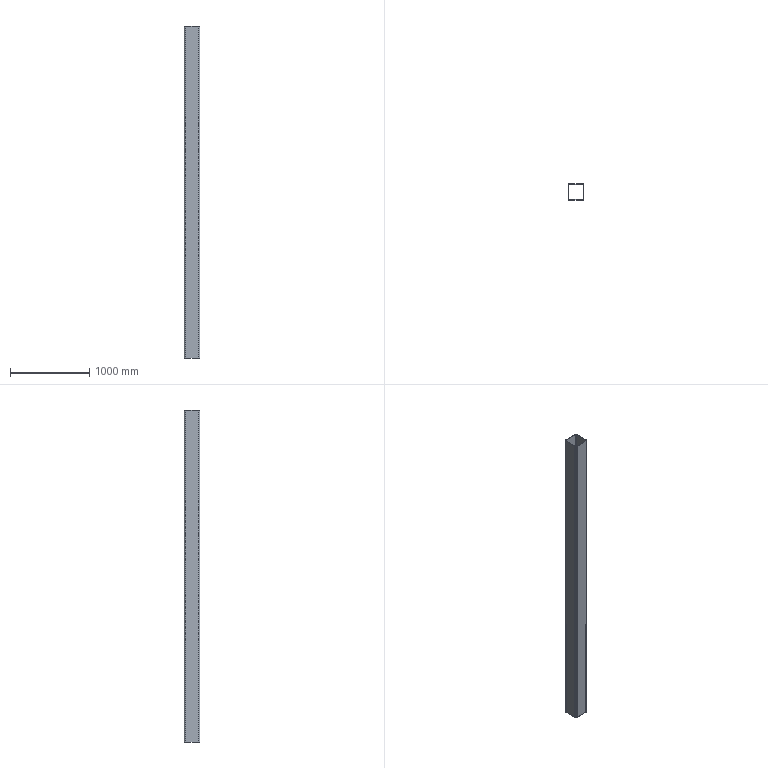Part | SolidWorks | features Extrusion 1 | 1 solid | 18 faces | box 200 x 200 x 4180 mm | volume 15674075 mm3 | plane 10 | cylinder 8 | commonest cylinder face diameters 30 x4 40 x4
STEP:
#1=CARTESIAN_POINT('',(-100.,-80.,4180.));
#2=VERTEX_POINT('',#1);
#3=CARTESIAN_POINT('',(-80.,-100.,4180.));
#4=VERTEX_POINT('',#3);
#5=CARTESIAN_POINT('',(-80.,-80.,4180.));
#6=DIRECTION('',(0.,0.,1.));
#7=DIRECTION('',(1.,0.,0.));
#8=AXIS2_PLACEMENT_3D('',#5,#6,#7);
#9=CIRCLE('',#8,20.);
#10=EDGE_CURVE('',#2,#4,#9,.T.);
#11=ORIENTED_EDGE('',*,*,#10,.T.);
#12=CARTESIAN_POINT('',(80.,-100.,4180.));
#13=VERTEX_POINT('',#12);
#14=CARTESIAN_POINT('',(-80.,-100.,4180.));
#15=DIRECTION('',(1.,0.,0.));
#16=VECTOR('',#15,1000.);
#17=LINE('',#14,#16);
#18=EDGE_CURVE('',#4,#13,#17,.T.);
#19=ORIENTED_EDGE('',*,*,#18,.T.);
#20=CARTESIAN_POINT('',(100.,-80.,4180.));
#21=VERTEX_POINT('',#20);
#22=CARTESIAN_POINT('',(80.,-80.,4180.));
#23=DIRECTION('',(0.,0.,1.));
#24=DIRECTION('',(1.,0.,0.));
#25=AXIS2_PLACEMENT_3D('',#22,#23,#24);
#26=CIRCLE('',#25,20.);
#27=EDGE_CURVE('',#13,#21,#26,.T.);
#28=ORIENTED_EDGE('',*,*,#27,.T.);
#29=CARTESIAN_POINT('',(100.,80.,4180.));
#30=VERTEX_POINT('',#29);
#31=CARTESIAN_POINT('',(100.,80.,4180.));
#32=DIRECTION('',(0.,1.,0.));
#33=VECTOR('',#32,1000.);
#34=LINE('',#31,#33);
#35=EDGE_CURVE('',#21,#30,#34,.T.);
#36=ORIENTED_EDGE('',*,*,#35,.T.);
#37=CARTESIAN_POINT('',(80.,100.,4180.));
#38=VERTEX_POINT('',#37);
#39=CARTESIAN_POINT('',(80.,80.,4180.));
#40=DIRECTION('',(0.,0.,1.));
#41=DIRECTION('',(-1.,0.,0.));
#42=AXIS2_PLACEMENT_3D('',#39,#40,#41);
#43=CIRCLE('',#42,20.);
#44=EDGE_CURVE('',#30,#38,#43,.T.);
#45=ORIENTED_EDGE('',*,*,#44,.T.);
#46=CARTESIAN_POINT('',(-80.,100.,4180.));
#47=VERTEX_POINT('',#46);
#48=CARTESIAN_POINT('',(-80.,100.,4180.));
#49=DIRECTION('',(-1.,0.,0.));
#50=VECTOR('',#49,1000.);
#51=LINE('',#48,#50);
#52=EDGE_CURVE('',#38,#47,#51,.T.);
#53=ORIENTED_EDGE('',*,*,#52,.T.);
#54=CARTESIAN_POINT('',(-100.,80.,4180.));
#55=VERTEX_POINT('',#54);
#56=CARTESIAN_POINT('',(-80.,80.,4180.));
#57=DIRECTION('',(0.,0.,1.));
#58=DIRECTION('',(1.,0.,0.));
#59=AXIS2_PLACEMENT_3D('',#56,#57,#58);
#60=CIRCLE('',#59,20.);
#61=EDGE_CURVE('',#47,#55,#60,.T.);
#62=ORIENTED_EDGE('',*,*,#61,.T.);
#63=CARTESIAN_POINT('',(-100.,80.,4180.));
#64=DIRECTION('',(0.,-1.,0.));
#65=VECTOR('',#64,1000.);
#66=LINE('',#63,#65);
#67=EDGE_CURVE('',#55,#2,#66,.T.);
#68=ORIENTED_EDGE('',*,*,#67,.T.);
#69=EDGE_LOOP('',(#11,#19,#28,#36,#45,#53,#62,#68));
#70=FACE_OUTER_BOUND('',#69,.T.);
#71=CARTESIAN_POINT('',(-95.,80.,4180.));
#72=VERTEX_POINT('',#71);
#73=CARTESIAN_POINT('',(-95.,-80.,4180.));
#74=VERTEX_POINT('',#73);
#75=CARTESIAN_POINT('',(-95.,80.,4180.));
#76=DIRECTION('',(0.,-1.,0.));
#77=VECTOR('',#76,1000.);
#78=LINE('',#75,#77);
#79=EDGE_CURVE('',#72,#74,#78,.T.);
#80=ORIENTED_EDGE('',*,*,#79,.F.);
#81=CARTESIAN_POINT('',(-80.,95.,4180.));
#82=VERTEX_POINT('',#81);
#83=CARTESIAN_POINT('',(-80.,80.,4180.));
#84=DIRECTION('',(0.,0.,1.));
#85=DIRECTION('',(1.,0.,0.));
#86=AXIS2_PLACEMENT_3D('',#83,#84,#85);
#87=CIRCLE('',#86,15.);
#88=EDGE_CURVE('',#82,#72,#87,.T.);
#89=ORIENTED_EDGE('',*,*,#88,.F.);
#90=CARTESIAN_POINT('',(80.,95.,4180.));
#91=VERTEX_POINT('',#90);
#92=CARTESIAN_POINT('',(-80.,95.,4180.));
#93=DIRECTION('',(-1.,0.,0.));
#94=VECTOR('',#93,1000.);
#95=LINE('',#92,#94);
#96=EDGE_CURVE('',#91,#82,#95,.T.);
#97=ORIENTED_EDGE('',*,*,#96,.F.);
#98=CARTESIAN_POINT('',(95.,80.,4180.));
#99=VERTEX_POINT('',#98);
#100=CARTESIAN_POINT('',(80.,80.,4180.));
#101=DIRECTION('',(0.,0.,1.));
#102=DIRECTION('',(-1.,0.,0.));
#103=AXIS2_PLACEMENT_3D('',#100,#101,#102);
#104=CIRCLE('',#103,15.);
#105=EDGE_CURVE('',#99,#91,#104,.T.);
#106=ORIENTED_EDGE('',*,*,#105,.F.);
#107=CARTESIAN_POINT('',(95.,-80.,4180.));
#108=VERTEX_POINT('',#107);
#109=CARTESIAN_POINT('',(95.,80.,4180.));
#110=DIRECTION('',(0.,1.,0.));
#111=VECTOR('',#110,1000.);
#112=LINE('',#109,#111);
#113=EDGE_CURVE('',#108,#99,#112,.T.);
#114=ORIENTED_EDGE('',*,*,#113,.F.);
#115=CARTESIAN_POINT('',(80.,-95.,4180.));
#116=VERTEX_POINT('',#115);
#117=CARTESIAN_POINT('',(80.,-80.,4180.));
#118=DIRECTION('',(0.,0.,1.));
#119=DIRECTION('',(1.,0.,0.));
#120=AXIS2_PLACEMENT_3D('',#117,#118,#119);
#121=CIRCLE('',#120,15.);
#122=EDGE_CURVE('',#116,#108,#121,.T.);
#123=ORIENTED_EDGE('',*,*,#122,.F.);
#124=CARTESIAN_POINT('',(-80.,-95.,4180.));
#125=VERTEX_POINT('',#124);
#126=CARTESIAN_POINT('',(-80.,-95.,4180.));
#127=DIRECTION('',(1.,0.,0.));
#128=VECTOR('',#127,1000.);
#129=LINE('',#126,#128);
#130=EDGE_CURVE('',#125,#116,#129,.T.);
#131=ORIENTED_EDGE('',*,*,#130,.F.);
#132=CARTESIAN_POINT('',(-80.,-80.,4180.));
#133=DIRECTION('',(0.,0.,1.));
#134=DIRECTION('',(1.,0.,0.));
#135=AXIS2_PLACEMENT_3D('',#132,#133,#134);
#136=CIRCLE('',#135,15.);
#137=EDGE_CURVE('',#74,#125,#136,.T.);
#138=ORIENTED_EDGE('',*,*,#137,.F.);
#139=EDGE_LOOP('',(#80,#89,#97,#106,#114,#123,#131,#138));
#140=FACE_BOUND('',#139,.T.);
#141=CARTESIAN_POINT('',(-80.,-80.,4180.));
#142=DIRECTION('',(0.,0.,1.));
#143=DIRECTION('',(1.,0.,0.));
#144=AXIS2_PLACEMENT_3D('',#141,#142,#143);
#145=PLANE('',#144);
#146=ADVANCED_FACE('',(#70,#140),#145,.T.);
#147=CARTESIAN_POINT('',(-100.,-80.,0.));
#148=VERTEX_POINT('',#147);
#149=CARTESIAN_POINT('',(-80.,-100.,0.));
#150=VERTEX_POINT('',#149);
#151=CARTESIAN_POINT('',(-80.,-80.,0.));
#152=DIRECTION('',(0.,0.,1.));
#153=DIRECTION('',(1.,0.,0.));
#154=AXIS2_PLACEMENT_3D('',#151,#152,#153);
#155=CIRCLE('',#154,20.);
#156=EDGE_CURVE('',#148,#150,#155,.T.);
#157=ORIENTED_EDGE('',*,*,#156,.F.);
#158=CARTESIAN_POINT('',(-100.,80.,0.));
#159=VERTEX_POINT('',#158);
#160=CARTESIAN_POINT('',(-100.,80.,0.));
#161=DIRECTION('',(0.,-1.,0.));
#162=VECTOR('',#161,1000.);
#163=LINE('',#160,#162);
#164=EDGE_CURVE('',#159,#148,#163,.T.);
#165=ORIENTED_EDGE('',*,*,#164,.F.);
#166=CARTESIAN_POINT('',(-80.,100.,0.));
#167=VERTEX_POINT('',#166);
#168=CARTESIAN_POINT('',(-80.,80.,0.));
#169=DIRECTION('',(0.,0.,1.));
#170=DIRECTION('',(1.,0.,0.));
#171=AXIS2_PLACEMENT_3D('',#168,#169,#170);
#172=CIRCLE('',#171,20.);
#173=EDGE_CURVE('',#167,#159,#172,.T.);
#174=ORIENTED_EDGE('',*,*,#173,.F.);
#175=CARTESIAN_POINT('',(80.,100.,0.));
#176=VERTEX_POINT('',#175);
#177=CARTESIAN_POINT('',(-80.,100.,0.));
#178=DIRECTION('',(-1.,0.,0.));
#179=VECTOR('',#178,1000.);
#180=LINE('',#177,#179);
#181=EDGE_CURVE('',#176,#167,#180,.T.);
#182=ORIENTED_EDGE('',*,*,#181,.F.);
#183=CARTESIAN_POINT('',(100.,80.,0.));
#184=VERTEX_POINT('',#183);
#185=CARTESIAN_POINT('',(80.,80.,0.));
#186=DIRECTION('',(0.,0.,1.));
#187=DIRECTION('',(-1.,0.,0.));
#188=AXIS2_PLACEMENT_3D('',#185,#186,#187);
#189=CIRCLE('',#188,20.);
#190=EDGE_CURVE('',#184,#176,#189,.T.);
#191=ORIENTED_EDGE('',*,*,#190,.F.);
#192=CARTESIAN_POINT('',(100.,-80.,0.));
#193=VERTEX_POINT('',#192);
#194=CARTESIAN_POINT('',(100.,80.,0.));
#195=DIRECTION('',(0.,1.,0.));
#196=VECTOR('',#195,1000.);
#197=LINE('',#194,#196);
#198=EDGE_CURVE('',#193,#184,#197,.T.);
#199=ORIENTED_EDGE('',*,*,#198,.F.);
#200=CARTESIAN_POINT('',(80.,-100.,0.));
#201=VERTEX_POINT('',#200);
#202=CARTESIAN_POINT('',(80.,-80.,0.));
#203=DIRECTION('',(0.,0.,1.));
#204=DIRECTION('',(1.,0.,0.));
#205=AXIS2_PLACEMENT_3D('',#202,#203,#204);
#206=CIRCLE('',#205,20.);
#207=EDGE_CURVE('',#201,#193,#206,.T.);
#208=ORIENTED_EDGE('',*,*,#207,.F.);
#209=CARTESIAN_POINT('',(-80.,-100.,0.));
#210=DIRECTION('',(1.,0.,0.));
#211=VECTOR('',#210,1000.);
#212=LINE('',#209,#211);
#213=EDGE_CURVE('',#150,#201,#212,.T.);
#214=ORIENTED_EDGE('',*,*,#213,.F.);
#215=EDGE_LOOP('',(#157,#165,#174,#182,#191,#199,#208,#214));
#216=FACE_OUTER_BOUND('',#215,.T.);
#217=CARTESIAN_POINT('',(-80.,95.,0.));
#218=VERTEX_POINT('',#217);
#219=CARTESIAN_POINT('',(-95.,80.,0.));
#220=VERTEX_POINT('',#219);
#221=CARTESIAN_POINT('',(-80.,80.,0.));
#222=DIRECTION('',(0.,0.,1.));
#223=DIRECTION('',(1.,0.,0.));
#224=AXIS2_PLACEMENT_3D('',#221,#222,#223);
#225=CIRCLE('',#224,15.);
#226=EDGE_CURVE('',#218,#220,#225,.T.);
#227=ORIENTED_EDGE('',*,*,#226,.T.);
#228=CARTESIAN_POINT('',(-95.,-80.,0.));
#229=VERTEX_POINT('',#228);
#230=CARTESIAN_POINT('',(-95.,80.,0.));
#231=DIRECTION('',(0.,-1.,0.));
#232=VECTOR('',#231,1000.);
#233=LINE('',#230,#232);
#234=EDGE_CURVE('',#220,#229,#233,.T.);
#235=ORIENTED_EDGE('',*,*,#234,.T.);
#236=CARTESIAN_POINT('',(-80.,-95.,0.));
#237=VERTEX_POINT('',#236);
#238=CARTESIAN_POINT('',(-80.,-80.,0.));
#239=DIRECTION('',(0.,0.,1.));
#240=DIRECTION('',(1.,0.,0.));
#241=AXIS2_PLACEMENT_3D('',#238,#239,#240);
#242=CIRCLE('',#241,15.);
#243=EDGE_CURVE('',#229,#237,#242,.T.);
#244=ORIENTED_EDGE('',*,*,#243,.T.);
#245=CARTESIAN_POINT('',(80.,-95.,0.));
#246=VERTEX_POINT('',#245);
#247=CARTESIAN_POINT('',(-80.,-95.,0.));
#248=DIRECTION('',(1.,0.,0.));
#249=VECTOR('',#248,1000.);
#250=LINE('',#247,#249);
#251=EDGE_CURVE('',#237,#246,#250,.T.);
#252=ORIENTED_EDGE('',*,*,#251,.T.);
#253=CARTESIAN_POINT('',(95.,-80.,0.));
#254=VERTEX_POINT('',#253);
#255=CARTESIAN_POINT('',(80.,-80.,0.));
#256=DIRECTION('',(0.,0.,1.));
#257=DIRECTION('',(1.,0.,0.));
#258=AXIS2_PLACEMENT_3D('',#255,#256,#257);
#259=CIRCLE('',#258,15.);
#260=EDGE_CURVE('',#246,#254,#259,.T.);
#261=ORIENTED_EDGE('',*,*,#260,.T.);
#262=CARTESIAN_POINT('',(95.,80.,0.));
#263=VERTEX_POINT('',#262);
#264=CARTESIAN_POINT('',(95.,80.,0.));
#265=DIRECTION('',(0.,1.,0.));
#266=VECTOR('',#265,1000.);
#267=LINE('',#264,#266);
#268=EDGE_CURVE('',#254,#263,#267,.T.);
#269=ORIENTED_EDGE('',*,*,#268,.T.);
#270=CARTESIAN_POINT('',(80.,95.,0.));
#271=VERTEX_POINT('',#270);
#272=CARTESIAN_POINT('',(80.,80.,0.));
#273=DIRECTION('',(0.,0.,1.));
#274=DIRECTION('',(-1.,0.,0.));
#275=AXIS2_PLACEMENT_3D('',#272,#273,#274);
#276=CIRCLE('',#275,15.);
#277=EDGE_CURVE('',#263,#271,#276,.T.);
#278=ORIENTED_EDGE('',*,*,#277,.T.);
#279=CARTESIAN_POINT('',(-80.,95.,0.));
#280=DIRECTION('',(-1.,0.,0.));
#281=VECTOR('',#280,1000.);
#282=LINE('',#279,#281);
#283=EDGE_CURVE('',#271,#218,#282,.T.);
#284=ORIENTED_EDGE('',*,*,#283,.T.);
#285=EDGE_LOOP('',(#227,#235,#244,#252,#261,#269,#278,#284));
#286=FACE_BOUND('',#285,.T.);
#287=CARTESIAN_POINT('',(-80.,-80.,0.));
#288=DIRECTION('',(0.,0.,1.));
#289=DIRECTION('',(1.,0.,0.));
#290=AXIS2_PLACEMENT_3D('',#287,#288,#289);
#291=PLANE('',#290);
#292=ADVANCED_FACE('',(#216,#286),#291,.F.);
#293=ORIENTED_EDGE('',*,*,#156,.T.);
#294=CARTESIAN_POINT('',(-80.,-100.,4180.));
#295=DIRECTION('',(0.,0.,-1.));
#296=VECTOR('',#295,1000.);
#297=LINE('',#294,#296);
#298=EDGE_CURVE('',#4,#150,#297,.T.);
#299=ORIENTED_EDGE('',*,*,#298,.F.);
#300=ORIENTED_EDGE('',*,*,#10,.F.);
#301=CARTESIAN_POINT('',(-100.,-80.,4180.));
#302=DIRECTION('',(0.,0.,-1.));
#303=VECTOR('',#302,1000.);
#304=LINE('',#301,#303);
#305=EDGE_CURVE('',#2,#148,#304,.T.);
#306=ORIENTED_EDGE('',*,*,#305,.T.);
#307=EDGE_LOOP('',(#293,#299,#300,#306));
#308=FACE_OUTER_BOUND('',#307,.T.);
#309=CARTESIAN_POINT('',(-80.,-80.,4180.));
#310=DIRECTION('',(0.,0.,-1.));
#311=DIRECTION('',(-1.,0.,0.));
#312=AXIS2_PLACEMENT_3D('',#309,#310,#311);
#313=CYLINDRICAL_SURFACE('',#312,20.);
#314=ADVANCED_FACE('',(#308),#313,.T.);
#315=ORIENTED_EDGE('',*,*,#213,.T.);
#316=CARTESIAN_POINT('',(80.,-100.,4180.));
#317=DIRECTION('',(0.,0.,-1.));
#318=VECTOR('',#317,1000.);
#319=LINE('',#316,#318);
#320=EDGE_CURVE('',#13,#201,#319,.T.);
#321=ORIENTED_EDGE('',*,*,#320,.F.);
#322=ORIENTED_EDGE('',*,*,#18,.F.);
#323=ORIENTED_EDGE('',*,*,#298,.T.);
#324=EDGE_LOOP('',(#315,#321,#322,#323));
#325=FACE_OUTER_BOUND('',#324,.T.);
#326=CARTESIAN_POINT('',(-80.,-100.,4180.));
#327=DIRECTION('',(0.,1.,0.));
#328=DIRECTION('',(0.,0.,1.));
#329=AXIS2_PLACEMENT_3D('',#326,#327,#328);
#330=PLANE('',#329);
#331=ADVANCED_FACE('',(#325),#330,.F.);
#332=ORIENTED_EDGE('',*,*,#207,.T.);
#333=CARTESIAN_POINT('',(100.,-80.,4180.));
#334=DIRECTION('',(0.,0.,-1.));
#335=VECTOR('',#334,1000.);
#336=LINE('',#333,#335);
#337=EDGE_CURVE('',#21,#193,#336,.T.);
#338=ORIENTED_EDGE('',*,*,#337,.F.);
#339=ORIENTED_EDGE('',*,*,#27,.F.);
#340=ORIENTED_EDGE('',*,*,#320,.T.);
#341=EDGE_LOOP('',(#332,#338,#339,#340));
#342=FACE_OUTER_BOUND('',#341,.T.);
#343=CARTESIAN_POINT('',(80.,-80.,4180.));
#344=DIRECTION('',(0.,0.,-1.));
#345=DIRECTION('',(-1.,0.,0.));
#346=AXIS2_PLACEMENT_3D('',#343,#344,#345);
#347=CYLINDRICAL_SURFACE('',#346,20.);
#348=ADVANCED_FACE('',(#342),#347,.T.);
#349=ORIENTED_EDGE('',*,*,#198,.T.);
#350=CARTESIAN_POINT('',(100.,80.,4180.));
#351=DIRECTION('',(0.,0.,-1.));
#352=VECTOR('',#351,1000.);
#353=LINE('',#350,#352);
#354=EDGE_CURVE('',#30,#184,#353,.T.);
#355=ORIENTED_EDGE('',*,*,#354,.F.);
#356=ORIENTED_EDGE('',*,*,#35,.F.);
#357=ORIENTED_EDGE('',*,*,#337,.T.);
#358=EDGE_LOOP('',(#349,#355,#356,#357));
#359=FACE_OUTER_BOUND('',#358,.T.);
#360=CARTESIAN_POINT('',(100.,80.,4180.));
#361=DIRECTION('',(-1.,0.,0.));
#362=DIRECTION('',(0.,-1.,0.));
#363=AXIS2_PLACEMENT_3D('',#360,#361,#362);
#364=PLANE('',#363);
#365=ADVANCED_FACE('',(#359),#364,.F.);
#366=ORIENTED_EDGE('',*,*,#190,.T.);
#367=CARTESIAN_POINT('',(80.,100.,4180.));
#368=DIRECTION('',(0.,0.,-1.));
#369=VECTOR('',#368,1000.);
#370=LINE('',#367,#369);
#371=EDGE_CURVE('',#38,#176,#370,.T.);
#372=ORIENTED_EDGE('',*,*,#371,.F.);
#373=ORIENTED_EDGE('',*,*,#44,.F.);
#374=ORIENTED_EDGE('',*,*,#354,.T.);
#375=EDGE_LOOP('',(#366,#372,#373,#374));
#376=FACE_OUTER_BOUND('',#375,.T.);
#377=CARTESIAN_POINT('',(80.,80.,4180.));
#378=DIRECTION('',(0.,0.,-1.));
#379=DIRECTION('',(-1.,0.,0.));
#380=AXIS2_PLACEMENT_3D('',#377,#378,#379);
#381=CYLINDRICAL_SURFACE('',#380,20.);
#382=ADVANCED_FACE('',(#376),#381,.T.);
#383=ORIENTED_EDGE('',*,*,#181,.T.);
#384=CARTESIAN_POINT('',(-80.,100.,4180.));
#385=DIRECTION('',(0.,0.,-1.));
#386=VECTOR('',#385,1000.);
#387=LINE('',#384,#386);
#388=EDGE_CURVE('',#47,#167,#387,.T.);
#389=ORIENTED_EDGE('',*,*,#388,.F.);
#390=ORIENTED_EDGE('',*,*,#52,.F.);
#391=ORIENTED_EDGE('',*,*,#371,.T.);
#392=EDGE_LOOP('',(#383,#389,#390,#391));
#393=FACE_OUTER_BOUND('',#392,.T.);
#394=CARTESIAN_POINT('',(-80.,100.,4180.));
#395=DIRECTION('',(0.,-1.,0.));
#396=DIRECTION('',(0.,0.,-1.));
#397=AXIS2_PLACEMENT_3D('',#394,#395,#396);
#398=PLANE('',#397);
#399=ADVANCED_FACE('',(#393),#398,.F.);
#400=ORIENTED_EDGE('',*,*,#173,.T.);
#401=CARTESIAN_POINT('',(-100.,80.,4180.));
#402=DIRECTION('',(0.,0.,-1.));
#403=VECTOR('',#402,1000.);
#404=LINE('',#401,#403);
#405=EDGE_CURVE('',#55,#159,#404,.T.);
#406=ORIENTED_EDGE('',*,*,#405,.F.);
#407=ORIENTED_EDGE('',*,*,#61,.F.);
#408=ORIENTED_EDGE('',*,*,#388,.T.);
#409=EDGE_LOOP('',(#400,#406,#407,#408));
#410=FACE_OUTER_BOUND('',#409,.T.);
#411=CARTESIAN_POINT('',(-80.,80.,4180.));
#412=DIRECTION('',(0.,0.,-1.));
#413=DIRECTION('',(-1.,0.,0.));
#414=AXIS2_PLACEMENT_3D('',#411,#412,#413);
#415=CYLINDRICAL_SURFACE('',#414,20.);
#416=ADVANCED_FACE('',(#410),#415,.T.);
#417=ORIENTED_EDGE('',*,*,#164,.T.);
#418=ORIENTED_EDGE('',*,*,#305,.F.);
#419=ORIENTED_EDGE('',*,*,#67,.F.);
#420=ORIENTED_EDGE('',*,*,#405,.T.);
#421=EDGE_LOOP('',(#417,#418,#419,#420));
#422=FACE_OUTER_BOUND('',#421,.T.);
#423=CARTESIAN_POINT('',(-100.,80.,4180.));
#424=DIRECTION('',(1.,0.,0.));
#425=DIRECTION('',(0.,1.,0.));
#426=AXIS2_PLACEMENT_3D('',#423,#424,#425);
#427=PLANE('',#426);
#428=ADVANCED_FACE('',(#422),#427,.F.);
#429=ORIENTED_EDGE('',*,*,#226,.F.);
#430=CARTESIAN_POINT('',(-80.,95.,4180.));
#431=DIRECTION('',(0.,0.,-1.));
#432=VECTOR('',#431,1000.);
#433=LINE('',#430,#432);
#434=EDGE_CURVE('',#82,#218,#433,.T.);
#435=ORIENTED_EDGE('',*,*,#434,.F.);
#436=ORIENTED_EDGE('',*,*,#88,.T.);
#437=CARTESIAN_POINT('',(-95.,80.,4180.));
#438=DIRECTION('',(0.,0.,-1.));
#439=VECTOR('',#438,1000.);
#440=LINE('',#437,#439);
#441=EDGE_CURVE('',#72,#220,#440,.T.);
#442=ORIENTED_EDGE('',*,*,#441,.T.);
#443=EDGE_LOOP('',(#429,#435,#436,#442));
#444=FACE_OUTER_BOUND('',#443,.T.);
#445=CARTESIAN_POINT('',(-80.,80.,4180.));
#446=DIRECTION('',(0.,0.,-1.));
#447=DIRECTION('',(-1.,0.,0.));
#448=AXIS2_PLACEMENT_3D('',#445,#446,#447);
#449=CYLINDRICAL_SURFACE('',#448,15.);
#450=ADVANCED_FACE('',(#444),#449,.F.);
#451=ORIENTED_EDGE('',*,*,#234,.F.);
#452=ORIENTED_EDGE('',*,*,#441,.F.);
#453=ORIENTED_EDGE('',*,*,#79,.T.);
#454=CARTESIAN_POINT('',(-95.,-80.,4180.));
#455=DIRECTION('',(0.,0.,-1.));
#456=VECTOR('',#455,1000.);
#457=LINE('',#454,#456);
#458=EDGE_CURVE('',#74,#229,#457,.T.);
#459=ORIENTED_EDGE('',*,*,#458,.T.);
#460=EDGE_LOOP('',(#451,#452,#453,#459));
#461=FACE_OUTER_BOUND('',#460,.T.);
#462=CARTESIAN_POINT('',(-95.,80.,4180.));
#463=DIRECTION('',(1.,0.,0.));
#464=DIRECTION('',(0.,1.,0.));
#465=AXIS2_PLACEMENT_3D('',#462,#463,#464);
#466=PLANE('',#465);
#467=ADVANCED_FACE('',(#461),#466,.T.);
#468=ORIENTED_EDGE('',*,*,#243,.F.);
#469=ORIENTED_EDGE('',*,*,#458,.F.);
#470=ORIENTED_EDGE('',*,*,#137,.T.);
#471=CARTESIAN_POINT('',(-80.,-95.,4180.));
#472=DIRECTION('',(0.,0.,-1.));
#473=VECTOR('',#472,1000.);
#474=LINE('',#471,#473);
#475=EDGE_CURVE('',#125,#237,#474,.T.);
#476=ORIENTED_EDGE('',*,*,#475,.T.);
#477=EDGE_LOOP('',(#468,#469,#470,#476));
#478=FACE_OUTER_BOUND('',#477,.T.);
#479=CARTESIAN_POINT('',(-80.,-80.,4180.));
#480=DIRECTION('',(0.,0.,-1.));
#481=DIRECTION('',(-1.,0.,0.));
#482=AXIS2_PLACEMENT_3D('',#479,#480,#481);
#483=CYLINDRICAL_SURFACE('',#482,15.);
#484=ADVANCED_FACE('',(#478),#483,.F.);
#485=ORIENTED_EDGE('',*,*,#251,.F.);
#486=ORIENTED_EDGE('',*,*,#475,.F.);
#487=ORIENTED_EDGE('',*,*,#130,.T.);
#488=CARTESIAN_POINT('',(80.,-95.,4180.));
#489=DIRECTION('',(0.,0.,-1.));
#490=VECTOR('',#489,1000.);
#491=LINE('',#488,#490);
#492=EDGE_CURVE('',#116,#246,#491,.T.);
#493=ORIENTED_EDGE('',*,*,#492,.T.);
#494=EDGE_LOOP('',(#485,#486,#487,#493));
#495=FACE_OUTER_BOUND('',#494,.T.);
#496=CARTESIAN_POINT('',(-80.,-95.,4180.));
#497=DIRECTION('',(0.,1.,0.));
#498=DIRECTION('',(0.,0.,1.));
#499=AXIS2_PLACEMENT_3D('',#496,#497,#498);
#500=PLANE('',#499);
#501=ADVANCED_FACE('',(#495),#500,.T.);
#502=ORIENTED_EDGE('',*,*,#260,.F.);
#503=ORIENTED_EDGE('',*,*,#492,.F.);
#504=ORIENTED_EDGE('',*,*,#122,.T.);
#505=CARTESIAN_POINT('',(95.,-80.,4180.));
#506=DIRECTION('',(0.,0.,-1.));
#507=VECTOR('',#506,1000.);
#508=LINE('',#505,#507);
#509=EDGE_CURVE('',#108,#254,#508,.T.);
#510=ORIENTED_EDGE('',*,*,#509,.T.);
#511=EDGE_LOOP('',(#502,#503,#504,#510));
#512=FACE_OUTER_BOUND('',#511,.T.);
#513=CARTESIAN_POINT('',(80.,-80.,4180.));
#514=DIRECTION('',(0.,0.,-1.));
#515=DIRECTION('',(-1.,0.,0.));
#516=AXIS2_PLACEMENT_3D('',#513,#514,#515);
#517=CYLINDRICAL_SURFACE('',#516,15.);
#518=ADVANCED_FACE('',(#512),#517,.F.);
#519=ORIENTED_EDGE('',*,*,#268,.F.);
#520=ORIENTED_EDGE('',*,*,#509,.F.);
#521=ORIENTED_EDGE('',*,*,#113,.T.);
#522=CARTESIAN_POINT('',(95.,80.,4180.));
#523=DIRECTION('',(0.,0.,-1.));
#524=VECTOR('',#523,1000.);
#525=LINE('',#522,#524);
#526=EDGE_CURVE('',#99,#263,#525,.T.);
#527=ORIENTED_EDGE('',*,*,#526,.T.);
#528=EDGE_LOOP('',(#519,#520,#521,#527));
#529=FACE_OUTER_BOUND('',#528,.T.);
#530=CARTESIAN_POINT('',(95.,80.,4180.));
#531=DIRECTION('',(-1.,0.,0.));
#532=DIRECTION('',(0.,-1.,0.));
#533=AXIS2_PLACEMENT_3D('',#530,#531,#532);
#534=PLANE('',#533);
#535=ADVANCED_FACE('',(#529),#534,.T.);
#536=ORIENTED_EDGE('',*,*,#277,.F.);
#537=ORIENTED_EDGE('',*,*,#526,.F.);
#538=ORIENTED_EDGE('',*,*,#105,.T.);
#539=CARTESIAN_POINT('',(80.,95.,4180.));
#540=DIRECTION('',(0.,0.,-1.));
#541=VECTOR('',#540,1000.);
#542=LINE('',#539,#541);
#543=EDGE_CURVE('',#91,#271,#542,.T.);
#544=ORIENTED_EDGE('',*,*,#543,.T.);
#545=EDGE_LOOP('',(#536,#537,#538,#544));
#546=FACE_OUTER_BOUND('',#545,.T.);
#547=CARTESIAN_POINT('',(80.,80.,4180.));
#548=DIRECTION('',(0.,0.,-1.));
#549=DIRECTION('',(-1.,0.,0.));
#550=AXIS2_PLACEMENT_3D('',#547,#548,#549);
#551=CYLINDRICAL_SURFACE('',#550,15.);
#552=ADVANCED_FACE('',(#546),#551,.F.);
#553=ORIENTED_EDGE('',*,*,#283,.F.);
#554=ORIENTED_EDGE('',*,*,#543,.F.);
#555=ORIENTED_EDGE('',*,*,#96,.T.);
#556=ORIENTED_EDGE('',*,*,#434,.T.);
#557=EDGE_LOOP('',(#553,#554,#555,#556));
#558=FACE_OUTER_BOUND('',#557,.T.);
#559=CARTESIAN_POINT('',(-80.,95.,4180.));
#560=DIRECTION('',(0.,-1.,0.));
#561=DIRECTION('',(0.,0.,-1.));
#562=AXIS2_PLACEMENT_3D('',#559,#560,#561);
#563=PLANE('',#562);
#564=ADVANCED_FACE('',(#558),#563,.T.);
#565=CLOSED_SHELL('',(#146,#292,#314,#331,#348,#365,#382,#399,#416,#428,#450,#467,#484,#501,#518,#535,#552,#564));
#566=MANIFOLD_SOLID_BREP('',#565);
#567=CARTESIAN_POINT('',(0.,0.,0.));
#568=DIRECTION('',(0.,0.,1.));
#569=DIRECTION('',(1.,0.,0.));
#570=AXIS2_PLACEMENT_3D('',#567,#568,#569);
#571=(LENGTH_UNIT()NAMED_UNIT(*)SI_UNIT(.MILLI.,.METRE.));
#572=UNCERTAINTY_MEASURE_WITH_UNIT(LENGTH_MEASURE(0.00001),#571,'','');
#573=(NAMED_UNIT(*)PLANE_ANGLE_UNIT()SI_UNIT($,.RADIAN.));
#574=(NAMED_UNIT(*)SI_UNIT($,.STERADIAN.)SOLID_ANGLE_UNIT());
#575=(GEOMETRIC_REPRESENTATION_CONTEXT(3)GLOBAL_UNCERTAINTY_ASSIGNED_CONTEXT((#572))GLOBAL_UNIT_ASSIGNED_CONTEXT((#571,#573,#574))REPRESENTATION_CONTEXT('',''));
#576=ADVANCED_BREP_SHAPE_REPRESENTATION('',(#566,#570),#575);